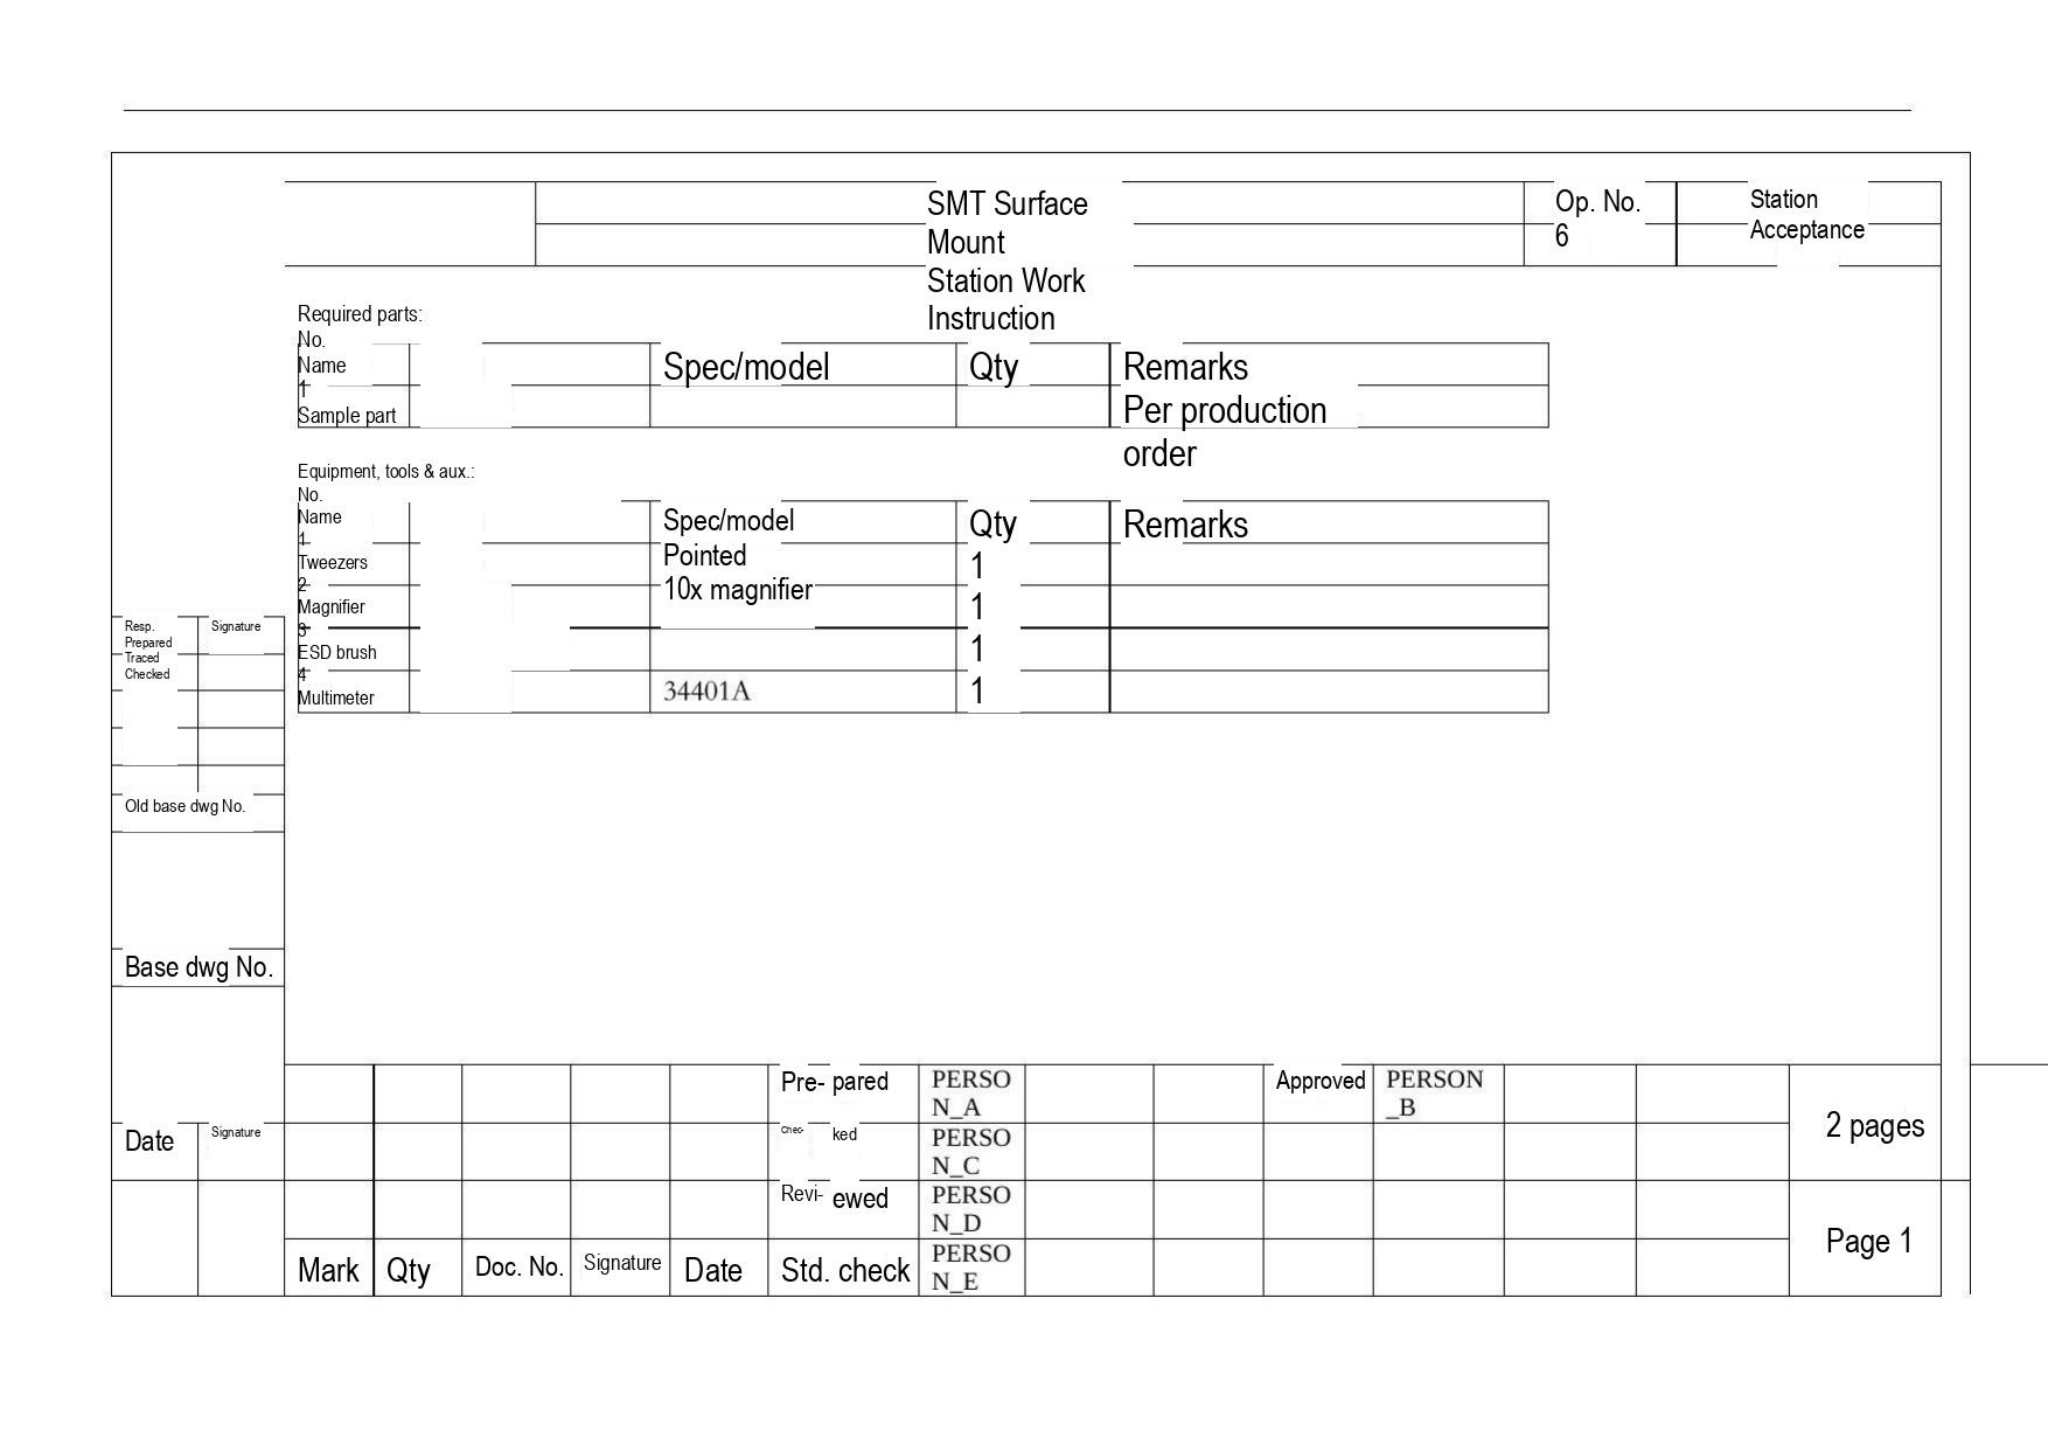SMT Surface Mount Station Work Instruction

Op. No. 6

Station Acceptance

Required parts:

| No. | Name | Spec/model | Qty | Remarks |
|---|---|---|---|---|
| 1 | Sample part | | | Per production order |

Equipment, tools & aux.:

| No. | Name | Spec/model | Qty | Remarks |
|---|---|---|---|---|
| 1 | Tweezers | Pointed | 1 | |
| 2 | Magnifier | 10x magnifier | 1 | |
| 3 | ESD brush | | 1 | |
| 4 | Multimeter | 34401A | 1 | |

| Resp. | Signature |
|---|---|
| Prepared | |
| Traced | |
| Checked | |

Old base dwg No.

Base dwg No.

| Date | Signature |
|---|---|

| | | | | | Prepared | PERSON_A | | | Approved | PERSON_B | | | 2 pages |
|---|---|---|---|---|---|---|---|---|---|---|---|---|---|
| | | | | | Checked | PERSON_C | | | | | | | |
| | | | | | Reviewed | PERSON_D | | | | | | | Page 1 |
| Mark | Qty | Doc. No. | Signature | Date | Std. check | PERSON_E | | | | | | | |
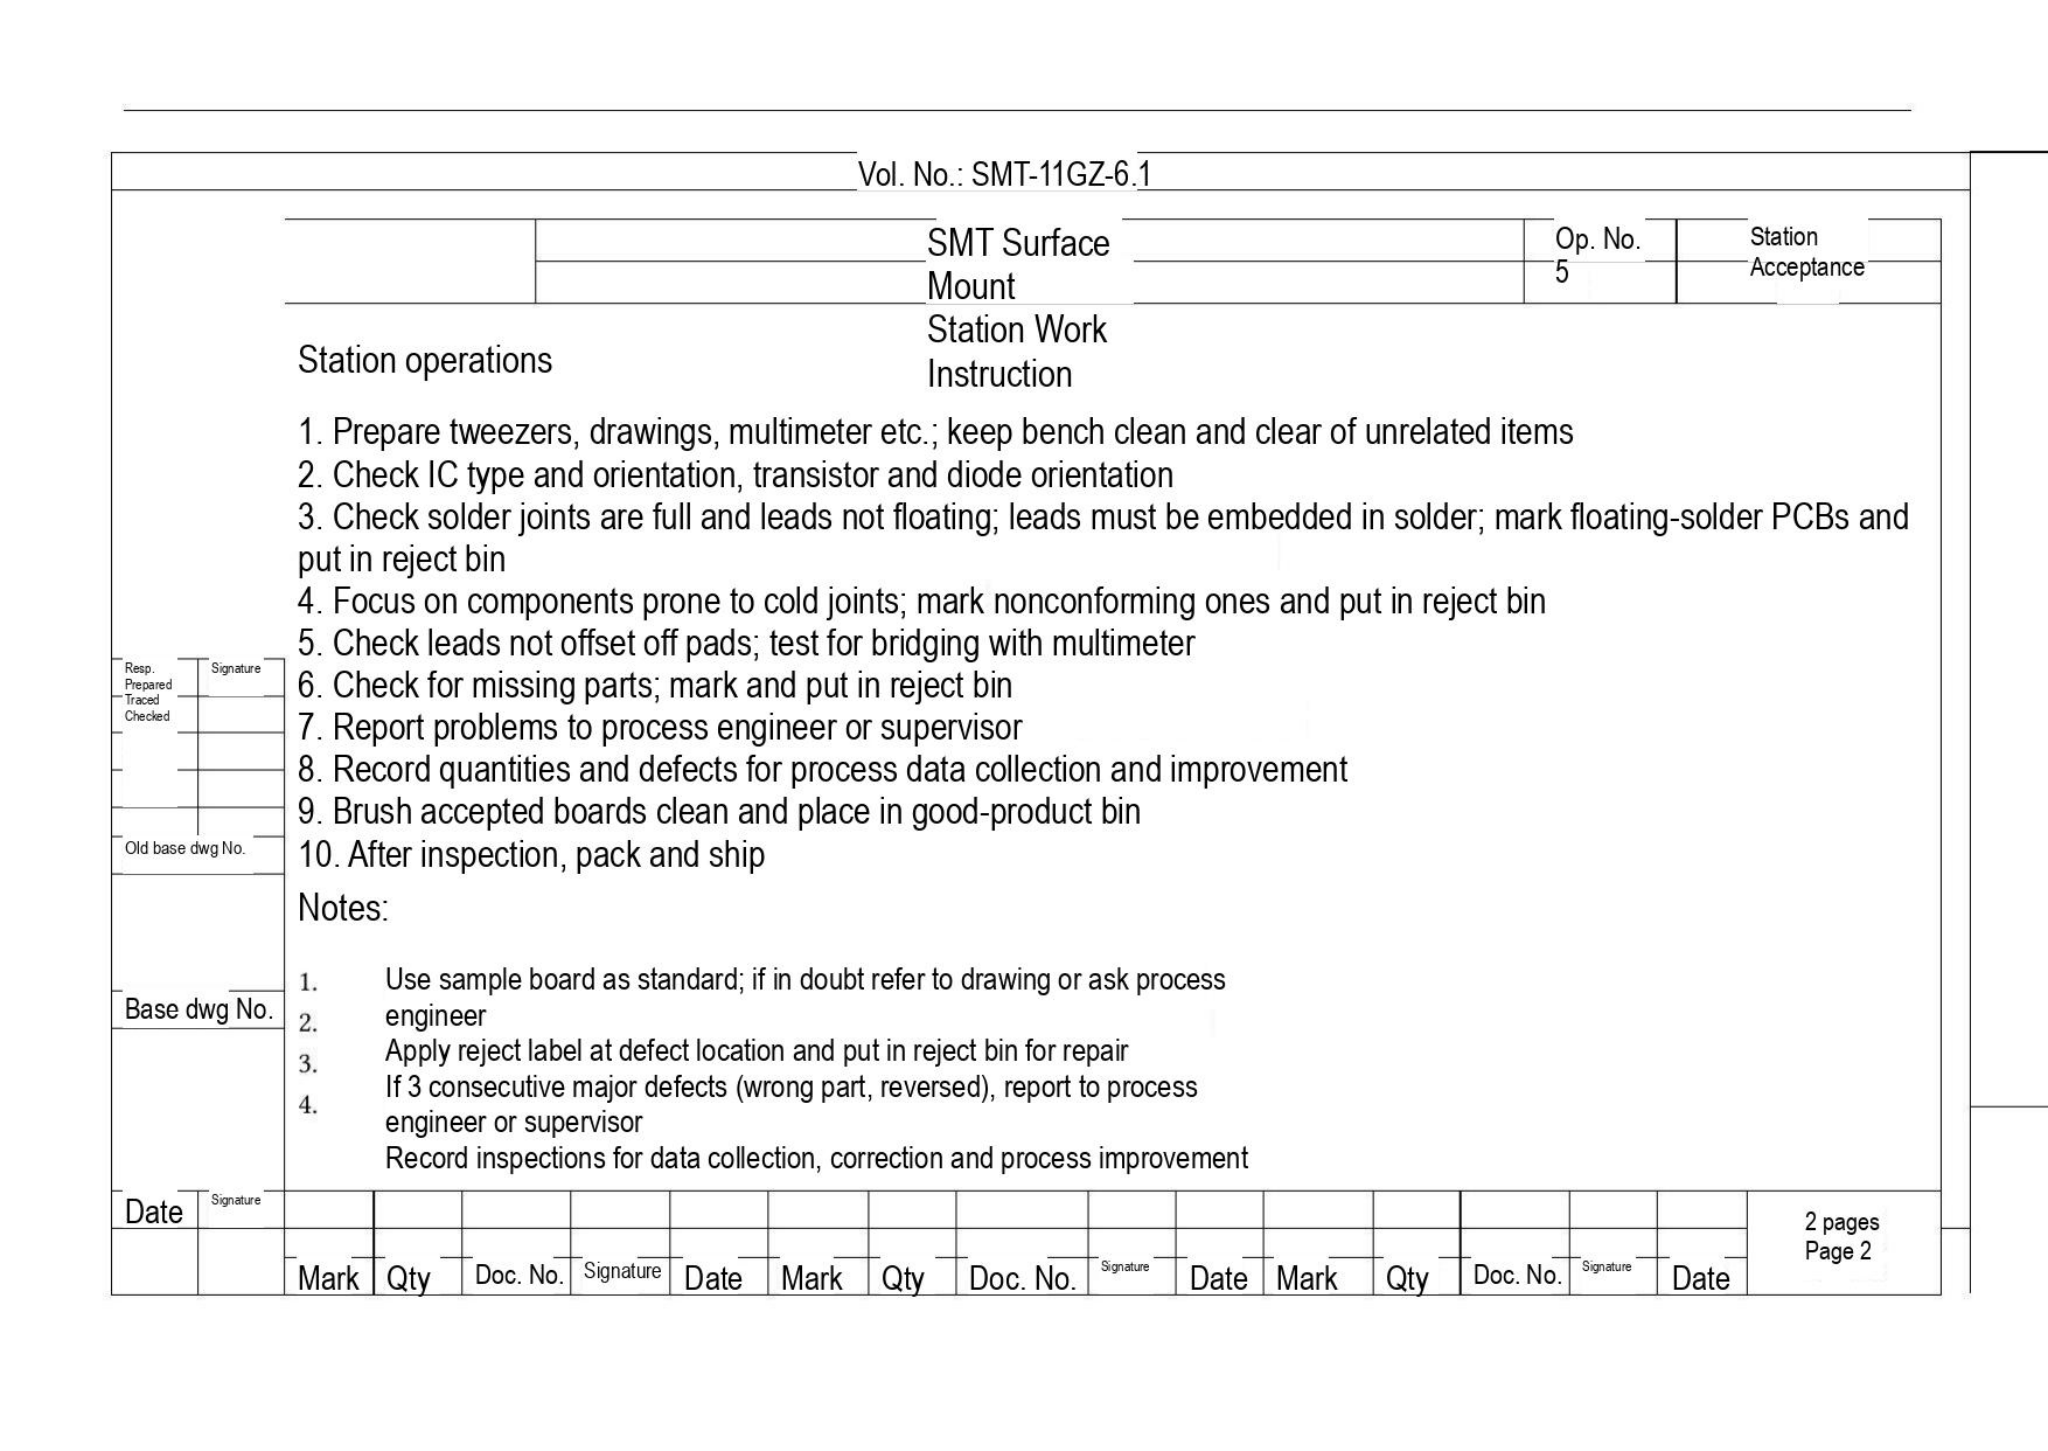Vol. No.: SMT-11GZ-6.1

| | SMT Surface Mount Station Work Instruction | Op. No. 5 | Station Acceptance |
|---|---|---|---|

Station operations

1. Prepare tweezers, drawings, multimeter etc.; keep bench clean and clear of unrelated items
2. Check IC type and orientation, transistor and diode orientation
3. Check solder joints are full and leads not floating; leads must be embedded in solder; mark floating-solder PCBs and put in reject bin
4. Focus on components prone to cold joints; mark nonconforming ones and put in reject bin
5. Check leads not offset off pads; test for bridging with multimeter
6. Check for missing parts; mark and put in reject bin
7. Report problems to process engineer or supervisor
8. Record quantities and defects for process data collection and improvement
9. Brush accepted boards clean and place in good-product bin
10. After inspection, pack and ship

Notes:

1. Use sample board as standard; if in doubt refer to drawing or ask process engineer
2. Apply reject label at defect location and put in reject bin for repair
3. If 3 consecutive major defects (wrong part, reversed), report to process engineer or supervisor
4. Record inspections for data collection, correction and process improvement

| Resp. | Signature |
|---|---|
| Prepared | |
| Traced | |
| Checked | |

Old base dwg No.

Base dwg No.

| Date | Signature |
|---|---|

| Mark | Qty | Doc. No. | Signature | Date | Mark | Qty | Doc. No. | Signature | Date | Mark | Qty | Doc. No. | Signature | Date | 2 pages Page 2 |
|---|---|---|---|---|---|---|---|---|---|---|---|---|---|---|---|